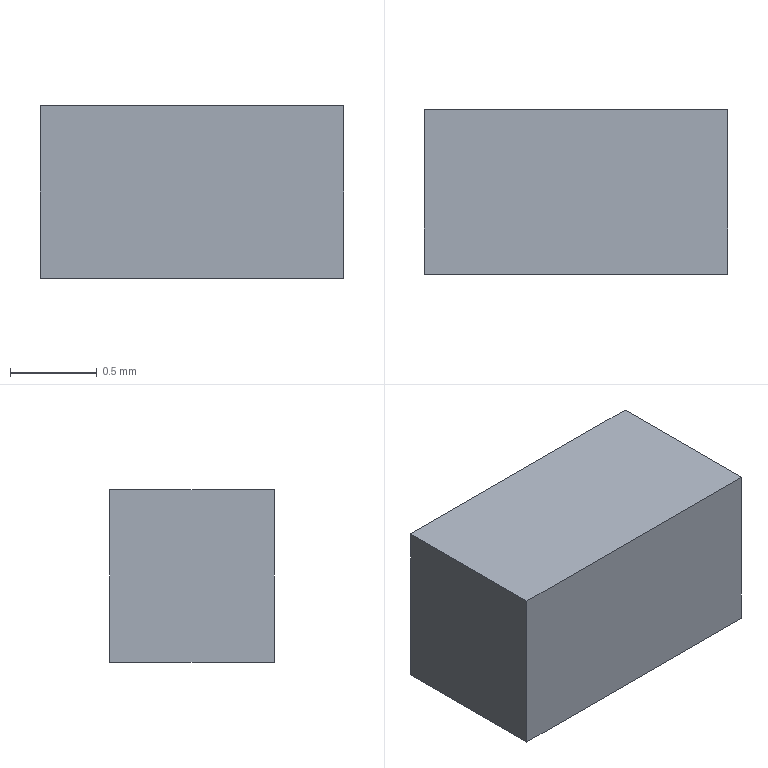Part | Creo | 1 solid | 6 faces | box 1.75 x 0.95 x 0.9956 mm | volume 1.655 mm3 | plane 6
STEP:
#1=CARTESIAN_POINT('',(0.,0.,0.));
#2=DIRECTION('',(0.,0.,1.));
#3=DIRECTION('',(1.,0.,0.));
#4=AXIS2_PLACEMENT_3D('',#1,#2,#3);
#5=CARTESIAN_POINT('',(-0.825,-0.425,0.));
#6=VERTEX_POINT('',#5);
#7=CARTESIAN_POINT('',(0.925,-0.425,0.));
#8=VERTEX_POINT('',#7);
#9=CARTESIAN_POINT('',(-0.825,-0.425,0.));
#10=DIRECTION('',(1.,0.,0.));
#11=VECTOR('',#10,1.75);
#12=LINE('',#9,#11);
#13=EDGE_CURVE('',#6,#8,#12,.T.);
#14=ORIENTED_EDGE('',*,*,#13,.T.);
#15=CARTESIAN_POINT('',(0.925,0.525,0.));
#16=VERTEX_POINT('',#15);
#17=CARTESIAN_POINT('',(0.925,-0.425,0.));
#18=DIRECTION('',(0.,1.,0.));
#19=VECTOR('',#18,0.95);
#20=LINE('',#17,#19);
#21=EDGE_CURVE('',#8,#16,#20,.T.);
#22=ORIENTED_EDGE('',*,*,#21,.T.);
#23=CARTESIAN_POINT('',(-0.825,0.525,0.));
#24=VERTEX_POINT('',#23);
#25=CARTESIAN_POINT('',(0.925,0.525,0.));
#26=DIRECTION('',(-1.,0.,0.));
#27=VECTOR('',#26,1.75);
#28=LINE('',#25,#27);
#29=EDGE_CURVE('',#16,#24,#28,.T.);
#30=ORIENTED_EDGE('',*,*,#29,.T.);
#31=CARTESIAN_POINT('',(-0.825,0.525,0.));
#32=DIRECTION('',(0.,-1.,0.));
#33=VECTOR('',#32,0.95);
#34=LINE('',#31,#33);
#35=EDGE_CURVE('',#24,#6,#34,.T.);
#36=ORIENTED_EDGE('',*,*,#35,.T.);
#37=EDGE_LOOP('',(#14,#22,#30,#36));
#38=FACE_OUTER_BOUND('',#37,.F.);
#39=CARTESIAN_POINT('',(0.,0.,0.));
#40=DIRECTION('',(0.,0.,1.));
#41=DIRECTION('',(1.,0.,0.));
#42=AXIS2_PLACEMENT_3D('',#39,#40,#41);
#43=PLANE('',#42);
#44=ADVANCED_FACE('',(#38),#43,.F.);
#45=ORIENTED_EDGE('',*,*,#13,.F.);
#46=CARTESIAN_POINT('',(-0.825,-0.425,0.9956));
#47=VERTEX_POINT('',#46);
#48=CARTESIAN_POINT('',(-0.825,-0.425,0.));
#49=DIRECTION('',(0.,0.,1.));
#50=VECTOR('',#49,0.9956);
#51=LINE('',#48,#50);
#52=EDGE_CURVE('',#6,#47,#51,.T.);
#53=ORIENTED_EDGE('',*,*,#52,.T.);
#54=CARTESIAN_POINT('',(0.925,-0.425,0.9956));
#55=VERTEX_POINT('',#54);
#56=CARTESIAN_POINT('',(-0.825,-0.425,0.9956));
#57=DIRECTION('',(1.,0.,0.));
#58=VECTOR('',#57,1.75);
#59=LINE('',#56,#58);
#60=EDGE_CURVE('',#47,#55,#59,.T.);
#61=ORIENTED_EDGE('',*,*,#60,.T.);
#62=CARTESIAN_POINT('',(0.925,-0.425,0.));
#63=DIRECTION('',(0.,0.,1.));
#64=VECTOR('',#63,0.9956);
#65=LINE('',#62,#64);
#66=EDGE_CURVE('',#8,#55,#65,.T.);
#67=ORIENTED_EDGE('',*,*,#66,.F.);
#68=EDGE_LOOP('',(#45,#53,#61,#67));
#69=FACE_OUTER_BOUND('',#68,.F.);
#70=CARTESIAN_POINT('',(-0.825,-0.425,0.));
#71=DIRECTION('',(0.,-1.,0.));
#72=DIRECTION('',(1.,0.,0.));
#73=AXIS2_PLACEMENT_3D('',#70,#71,#72);
#74=PLANE('',#73);
#75=ADVANCED_FACE('',(#69),#74,.T.);
#76=ORIENTED_EDGE('',*,*,#35,.F.);
#77=CARTESIAN_POINT('',(-0.825,0.525,0.9956));
#78=VERTEX_POINT('',#77);
#79=CARTESIAN_POINT('',(-0.825,0.525,0.));
#80=DIRECTION('',(0.,0.,1.));
#81=VECTOR('',#80,0.9956);
#82=LINE('',#79,#81);
#83=EDGE_CURVE('',#24,#78,#82,.T.);
#84=ORIENTED_EDGE('',*,*,#83,.T.);
#85=CARTESIAN_POINT('',(-0.825,0.525,0.9956));
#86=DIRECTION('',(0.,-1.,0.));
#87=VECTOR('',#86,0.95);
#88=LINE('',#85,#87);
#89=EDGE_CURVE('',#78,#47,#88,.T.);
#90=ORIENTED_EDGE('',*,*,#89,.T.);
#91=ORIENTED_EDGE('',*,*,#52,.F.);
#92=EDGE_LOOP('',(#76,#84,#90,#91));
#93=FACE_OUTER_BOUND('',#92,.F.);
#94=CARTESIAN_POINT('',(-0.825,0.525,0.));
#95=DIRECTION('',(-1.,0.,0.));
#96=DIRECTION('',(0.,-1.,0.));
#97=AXIS2_PLACEMENT_3D('',#94,#95,#96);
#98=PLANE('',#97);
#99=ADVANCED_FACE('',(#93),#98,.T.);
#100=ORIENTED_EDGE('',*,*,#29,.F.);
#101=CARTESIAN_POINT('',(0.925,0.525,0.9956));
#102=VERTEX_POINT('',#101);
#103=CARTESIAN_POINT('',(0.925,0.525,0.));
#104=DIRECTION('',(0.,0.,1.));
#105=VECTOR('',#104,0.9956);
#106=LINE('',#103,#105);
#107=EDGE_CURVE('',#16,#102,#106,.T.);
#108=ORIENTED_EDGE('',*,*,#107,.T.);
#109=CARTESIAN_POINT('',(0.925,0.525,0.9956));
#110=DIRECTION('',(-1.,0.,0.));
#111=VECTOR('',#110,1.75);
#112=LINE('',#109,#111);
#113=EDGE_CURVE('',#102,#78,#112,.T.);
#114=ORIENTED_EDGE('',*,*,#113,.T.);
#115=ORIENTED_EDGE('',*,*,#83,.F.);
#116=EDGE_LOOP('',(#100,#108,#114,#115));
#117=FACE_OUTER_BOUND('',#116,.F.);
#118=CARTESIAN_POINT('',(0.925,0.525,0.));
#119=DIRECTION('',(0.,1.,0.));
#120=DIRECTION('',(-1.,0.,0.));
#121=AXIS2_PLACEMENT_3D('',#118,#119,#120);
#122=PLANE('',#121);
#123=ADVANCED_FACE('',(#117),#122,.T.);
#124=ORIENTED_EDGE('',*,*,#21,.F.);
#125=ORIENTED_EDGE('',*,*,#66,.T.);
#126=CARTESIAN_POINT('',(0.925,-0.425,0.9956));
#127=DIRECTION('',(0.,1.,0.));
#128=VECTOR('',#127,0.95);
#129=LINE('',#126,#128);
#130=EDGE_CURVE('',#55,#102,#129,.T.);
#131=ORIENTED_EDGE('',*,*,#130,.T.);
#132=ORIENTED_EDGE('',*,*,#107,.F.);
#133=EDGE_LOOP('',(#124,#125,#131,#132));
#134=FACE_OUTER_BOUND('',#133,.F.);
#135=CARTESIAN_POINT('',(0.925,-0.425,0.));
#136=DIRECTION('',(1.,0.,0.));
#137=DIRECTION('',(0.,1.,0.));
#138=AXIS2_PLACEMENT_3D('',#135,#136,#137);
#139=PLANE('',#138);
#140=ADVANCED_FACE('',(#134),#139,.T.);
#141=ORIENTED_EDGE('',*,*,#60,.F.);
#142=ORIENTED_EDGE('',*,*,#89,.F.);
#143=ORIENTED_EDGE('',*,*,#113,.F.);
#144=ORIENTED_EDGE('',*,*,#130,.F.);
#145=EDGE_LOOP('',(#141,#142,#143,#144));
#146=FACE_OUTER_BOUND('',#145,.F.);
#147=CARTESIAN_POINT('',(0.,0.,0.9956));
#148=DIRECTION('',(0.,0.,1.));
#149=DIRECTION('',(1.,0.,0.));
#150=AXIS2_PLACEMENT_3D('',#147,#148,#149);
#151=PLANE('',#150);
#152=ADVANCED_FACE('',(#146),#151,.T.);
#153=CLOSED_SHELL('',(#44,#75,#99,#123,#140,#152));
#154=MANIFOLD_SOLID_BREP('',#153);
#155=(LENGTH_UNIT()NAMED_UNIT(*)SI_UNIT(.MILLI.,.METRE.));
#156=UNCERTAINTY_MEASURE_WITH_UNIT(LENGTH_MEASURE(0.0002226),#155,'','');
#157=(NAMED_UNIT(*)PLANE_ANGLE_UNIT()SI_UNIT($,.RADIAN.));
#158=PLANE_ANGLE_MEASURE_WITH_UNIT(PLANE_ANGLE_MEASURE(0.01745),#157);
#159=(CONVERSION_BASED_UNIT('DEGREE',#158)NAMED_UNIT(*)PLANE_ANGLE_UNIT());
#160=(NAMED_UNIT(*)SI_UNIT($,.STERADIAN.)SOLID_ANGLE_UNIT());
#161=(GEOMETRIC_REPRESENTATION_CONTEXT(3)GLOBAL_UNCERTAINTY_ASSIGNED_CONTEXT((#156))GLOBAL_UNIT_ASSIGNED_CONTEXT((#155,#159,#160))REPRESENTATION_CONTEXT('',''));
#162=ADVANCED_BREP_SHAPE_REPRESENTATION('',(#4,#154),#161);